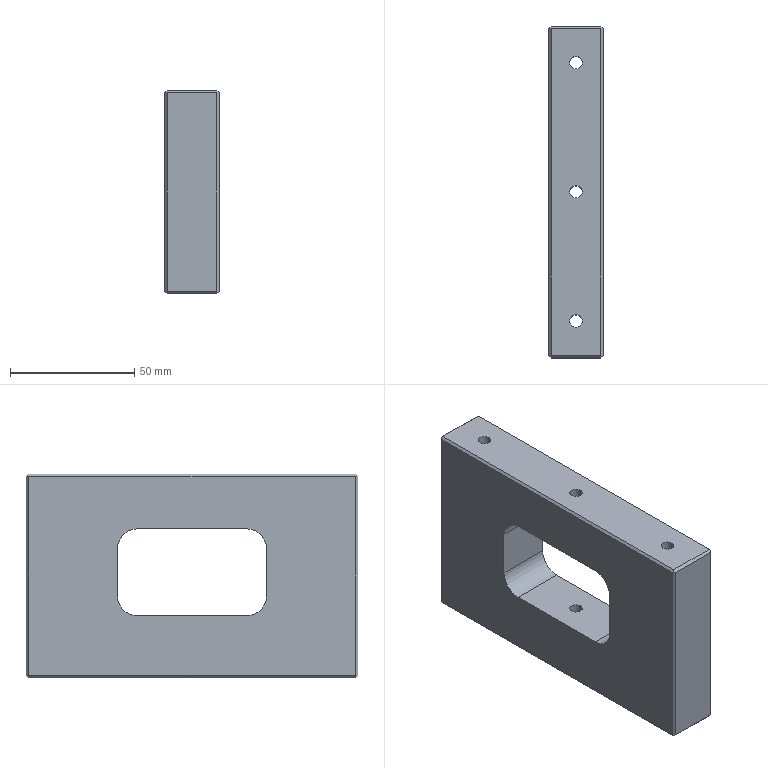Part | Creo | features DATUM PLANE 3, CURVE 2, CHAMFER 1, COORDINATE SYSTEM 1, CUT 1, PROTRUSION 1, ROUND 1 | 1 solid | 34 faces | box 22 x 133.5 x 82 mm | volume 191231 mm3 | plane 22 | cylinder 12 | commonest cylinder face diameters 5 x8 16 x4
STEP:
#1=CARTESIAN_POINT('',(0.,0.,0.));
#2=DIRECTION('',(0.,0.,1.));
#3=DIRECTION('',(1.,0.,0.));
#4=AXIS2_PLACEMENT_3D('',#1,#2,#3);
#5=CARTESIAN_POINT('',(-10.,-65.75,0.));
#6=VERTEX_POINT('',#5);
#7=CARTESIAN_POINT('',(-10.,65.75,0.));
#8=VERTEX_POINT('',#7);
#9=CARTESIAN_POINT('',(-10.,-65.75,0.));
#10=DIRECTION('',(0.,1.,0.));
#11=VECTOR('',#10,131.5);
#12=LINE('',#9,#11);
#13=EDGE_CURVE('',#6,#8,#12,.T.);
#14=ORIENTED_EDGE('',*,*,#13,.F.);
#15=CARTESIAN_POINT('',(10.,-65.75,0.));
#16=VERTEX_POINT('',#15);
#17=CARTESIAN_POINT('',(10.,-65.75,0.));
#18=DIRECTION('',(-1.,0.,0.));
#19=VECTOR('',#18,20.);
#20=LINE('',#17,#19);
#21=EDGE_CURVE('',#16,#6,#20,.T.);
#22=ORIENTED_EDGE('',*,*,#21,.F.);
#23=CARTESIAN_POINT('',(10.,65.75,0.));
#24=VERTEX_POINT('',#23);
#25=CARTESIAN_POINT('',(10.,65.75,0.));
#26=DIRECTION('',(0.,-1.,0.));
#27=VECTOR('',#26,131.5);
#28=LINE('',#25,#27);
#29=EDGE_CURVE('',#24,#16,#28,.T.);
#30=ORIENTED_EDGE('',*,*,#29,.F.);
#31=CARTESIAN_POINT('',(-10.,65.75,0.));
#32=DIRECTION('',(1.,0.,0.));
#33=VECTOR('',#32,20.);
#34=LINE('',#31,#33);
#35=EDGE_CURVE('',#8,#24,#34,.T.);
#36=ORIENTED_EDGE('',*,*,#35,.F.);
#37=EDGE_LOOP('',(#14,#22,#30,#36));
#38=FACE_OUTER_BOUND('',#37,.F.);
#39=CARTESIAN_POINT('',(2.5,0.,0.));
#40=VERTEX_POINT('',#39);
#41=CARTESIAN_POINT('',(-2.5,0.,0.));
#42=VERTEX_POINT('',#41);
#43=CARTESIAN_POINT('',(0.,0.,0.));
#44=DIRECTION('',(0.,0.,-1.));
#45=DIRECTION('',(1.,0.,0.));
#46=AXIS2_PLACEMENT_3D('',#43,#44,#45);
#47=CIRCLE('',#46,2.5);
#48=EDGE_CURVE('',#40,#42,#47,.T.);
#49=ORIENTED_EDGE('',*,*,#48,.T.);
#50=CARTESIAN_POINT('',(0.,0.,0.));
#51=DIRECTION('',(0.,0.,-1.));
#52=DIRECTION('',(-1.,0.,0.));
#53=AXIS2_PLACEMENT_3D('',#50,#51,#52);
#54=CIRCLE('',#53,2.5);
#55=EDGE_CURVE('',#42,#40,#54,.T.);
#56=ORIENTED_EDGE('',*,*,#55,.T.);
#57=EDGE_LOOP('',(#49,#56));
#58=FACE_BOUND('',#57,.F.);
#59=CARTESIAN_POINT('',(2.5,-52.,0.));
#60=VERTEX_POINT('',#59);
#61=CARTESIAN_POINT('',(-2.5,-52.,0.));
#62=VERTEX_POINT('',#61);
#63=CARTESIAN_POINT('',(0.,-52.,0.));
#64=DIRECTION('',(0.,0.,-1.));
#65=DIRECTION('',(1.,0.,0.));
#66=AXIS2_PLACEMENT_3D('',#63,#64,#65);
#67=CIRCLE('',#66,2.5);
#68=EDGE_CURVE('',#60,#62,#67,.T.);
#69=ORIENTED_EDGE('',*,*,#68,.T.);
#70=CARTESIAN_POINT('',(0.,-52.,0.));
#71=DIRECTION('',(0.,0.,-1.));
#72=DIRECTION('',(-1.,0.,0.));
#73=AXIS2_PLACEMENT_3D('',#70,#71,#72);
#74=CIRCLE('',#73,2.5);
#75=EDGE_CURVE('',#62,#60,#74,.T.);
#76=ORIENTED_EDGE('',*,*,#75,.T.);
#77=EDGE_LOOP('',(#69,#76));
#78=FACE_BOUND('',#77,.F.);
#79=CARTESIAN_POINT('',(2.5,52.,0.));
#80=VERTEX_POINT('',#79);
#81=CARTESIAN_POINT('',(-2.5,52.,0.));
#82=VERTEX_POINT('',#81);
#83=CARTESIAN_POINT('',(0.,52.,0.));
#84=DIRECTION('',(0.,0.,-1.));
#85=DIRECTION('',(1.,0.,0.));
#86=AXIS2_PLACEMENT_3D('',#83,#84,#85);
#87=CIRCLE('',#86,2.5);
#88=EDGE_CURVE('',#80,#82,#87,.T.);
#89=ORIENTED_EDGE('',*,*,#88,.T.);
#90=CARTESIAN_POINT('',(0.,52.,0.));
#91=DIRECTION('',(0.,0.,-1.));
#92=DIRECTION('',(-1.,0.,0.));
#93=AXIS2_PLACEMENT_3D('',#90,#91,#92);
#94=CIRCLE('',#93,2.5);
#95=EDGE_CURVE('',#82,#80,#94,.T.);
#96=ORIENTED_EDGE('',*,*,#95,.T.);
#97=EDGE_LOOP('',(#89,#96));
#98=FACE_BOUND('',#97,.F.);
#99=CARTESIAN_POINT('',(0.,0.,0.));
#100=DIRECTION('',(0.,0.,1.));
#101=DIRECTION('',(1.,0.,0.));
#102=AXIS2_PLACEMENT_3D('',#99,#100,#101);
#103=PLANE('',#102);
#104=ADVANCED_FACE('',(#38,#58,#78,#98),#103,.F.);
#105=ORIENTED_EDGE('',*,*,#88,.F.);
#106=CARTESIAN_POINT('',(2.5,52.,82.));
#107=VERTEX_POINT('',#106);
#108=CARTESIAN_POINT('',(2.5,52.,0.));
#109=DIRECTION('',(0.,0.,1.));
#110=VECTOR('',#109,82.);
#111=LINE('',#108,#110);
#112=EDGE_CURVE('',#80,#107,#111,.T.);
#113=ORIENTED_EDGE('',*,*,#112,.T.);
#114=CARTESIAN_POINT('',(-2.5,52.,82.));
#115=VERTEX_POINT('',#114);
#116=CARTESIAN_POINT('',(0.,52.,82.));
#117=DIRECTION('',(0.,0.,-1.));
#118=DIRECTION('',(1.,0.,0.));
#119=AXIS2_PLACEMENT_3D('',#116,#117,#118);
#120=CIRCLE('',#119,2.5);
#121=EDGE_CURVE('',#107,#115,#120,.T.);
#122=ORIENTED_EDGE('',*,*,#121,.T.);
#123=CARTESIAN_POINT('',(-2.5,52.,0.));
#124=DIRECTION('',(0.,0.,1.));
#125=VECTOR('',#124,82.);
#126=LINE('',#123,#125);
#127=EDGE_CURVE('',#82,#115,#126,.T.);
#128=ORIENTED_EDGE('',*,*,#127,.F.);
#129=EDGE_LOOP('',(#105,#113,#122,#128));
#130=FACE_OUTER_BOUND('',#129,.F.);
#131=CARTESIAN_POINT('',(0.,52.,0.));
#132=DIRECTION('',(0.,0.,1.));
#133=DIRECTION('',(1.,0.,0.));
#134=AXIS2_PLACEMENT_3D('',#131,#132,#133);
#135=CYLINDRICAL_SURFACE('',#134,2.5);
#136=ADVANCED_FACE('',(#130),#135,.F.);
#137=ORIENTED_EDGE('',*,*,#95,.F.);
#138=ORIENTED_EDGE('',*,*,#127,.T.);
#139=CARTESIAN_POINT('',(0.,52.,82.));
#140=DIRECTION('',(0.,0.,-1.));
#141=DIRECTION('',(-1.,0.,0.));
#142=AXIS2_PLACEMENT_3D('',#139,#140,#141);
#143=CIRCLE('',#142,2.5);
#144=EDGE_CURVE('',#115,#107,#143,.T.);
#145=ORIENTED_EDGE('',*,*,#144,.T.);
#146=ORIENTED_EDGE('',*,*,#112,.F.);
#147=EDGE_LOOP('',(#137,#138,#145,#146));
#148=FACE_OUTER_BOUND('',#147,.F.);
#149=CARTESIAN_POINT('',(0.,52.,0.));
#150=DIRECTION('',(0.,0.,1.));
#151=DIRECTION('',(1.,0.,0.));
#152=AXIS2_PLACEMENT_3D('',#149,#150,#151);
#153=CYLINDRICAL_SURFACE('',#152,2.5);
#154=ADVANCED_FACE('',(#148),#153,.F.);
#155=CARTESIAN_POINT('',(10.,65.75,82.));
#156=VERTEX_POINT('',#155);
#157=CARTESIAN_POINT('',(-10.,65.75,82.));
#158=VERTEX_POINT('',#157);
#159=CARTESIAN_POINT('',(10.,65.75,82.));
#160=DIRECTION('',(-1.,0.,0.));
#161=VECTOR('',#160,20.);
#162=LINE('',#159,#161);
#163=EDGE_CURVE('',#156,#158,#162,.T.);
#164=ORIENTED_EDGE('',*,*,#163,.F.);
#165=CARTESIAN_POINT('',(10.,-65.75,82.));
#166=VERTEX_POINT('',#165);
#167=CARTESIAN_POINT('',(10.,-65.75,82.));
#168=DIRECTION('',(0.,1.,0.));
#169=VECTOR('',#168,131.5);
#170=LINE('',#167,#169);
#171=EDGE_CURVE('',#166,#156,#170,.T.);
#172=ORIENTED_EDGE('',*,*,#171,.F.);
#173=CARTESIAN_POINT('',(-10.,-65.75,82.));
#174=VERTEX_POINT('',#173);
#175=CARTESIAN_POINT('',(-10.,-65.75,82.));
#176=DIRECTION('',(1.,0.,0.));
#177=VECTOR('',#176,20.);
#178=LINE('',#175,#177);
#179=EDGE_CURVE('',#174,#166,#178,.T.);
#180=ORIENTED_EDGE('',*,*,#179,.F.);
#181=CARTESIAN_POINT('',(-10.,65.75,82.));
#182=DIRECTION('',(0.,-1.,0.));
#183=VECTOR('',#182,131.5);
#184=LINE('',#181,#183);
#185=EDGE_CURVE('',#158,#174,#184,.T.);
#186=ORIENTED_EDGE('',*,*,#185,.F.);
#187=EDGE_LOOP('',(#164,#172,#180,#186));
#188=FACE_OUTER_BOUND('',#187,.F.);
#189=CARTESIAN_POINT('',(2.5,0.,82.));
#190=VERTEX_POINT('',#189);
#191=CARTESIAN_POINT('',(-2.5,0.,82.));
#192=VERTEX_POINT('',#191);
#193=CARTESIAN_POINT('',(0.,0.,82.));
#194=DIRECTION('',(0.,0.,-1.));
#195=DIRECTION('',(1.,0.,0.));
#196=AXIS2_PLACEMENT_3D('',#193,#194,#195);
#197=CIRCLE('',#196,2.5);
#198=EDGE_CURVE('',#190,#192,#197,.T.);
#199=ORIENTED_EDGE('',*,*,#198,.F.);
#200=CARTESIAN_POINT('',(0.,0.,82.));
#201=DIRECTION('',(0.,0.,-1.));
#202=DIRECTION('',(-1.,0.,0.));
#203=AXIS2_PLACEMENT_3D('',#200,#201,#202);
#204=CIRCLE('',#203,2.5);
#205=EDGE_CURVE('',#192,#190,#204,.T.);
#206=ORIENTED_EDGE('',*,*,#205,.F.);
#207=EDGE_LOOP('',(#199,#206));
#208=FACE_BOUND('',#207,.F.);
#209=CARTESIAN_POINT('',(2.5,-52.,82.));
#210=VERTEX_POINT('',#209);
#211=CARTESIAN_POINT('',(-2.5,-52.,82.));
#212=VERTEX_POINT('',#211);
#213=CARTESIAN_POINT('',(0.,-52.,82.));
#214=DIRECTION('',(0.,0.,-1.));
#215=DIRECTION('',(1.,0.,0.));
#216=AXIS2_PLACEMENT_3D('',#213,#214,#215);
#217=CIRCLE('',#216,2.5);
#218=EDGE_CURVE('',#210,#212,#217,.T.);
#219=ORIENTED_EDGE('',*,*,#218,.F.);
#220=CARTESIAN_POINT('',(0.,-52.,82.));
#221=DIRECTION('',(0.,0.,-1.));
#222=DIRECTION('',(-1.,0.,0.));
#223=AXIS2_PLACEMENT_3D('',#220,#221,#222);
#224=CIRCLE('',#223,2.5);
#225=EDGE_CURVE('',#212,#210,#224,.T.);
#226=ORIENTED_EDGE('',*,*,#225,.F.);
#227=EDGE_LOOP('',(#219,#226));
#228=FACE_BOUND('',#227,.F.);
#229=ORIENTED_EDGE('',*,*,#121,.F.);
#230=ORIENTED_EDGE('',*,*,#144,.F.);
#231=EDGE_LOOP('',(#229,#230));
#232=FACE_BOUND('',#231,.F.);
#233=CARTESIAN_POINT('',(0.,0.,82.));
#234=DIRECTION('',(0.,0.,1.));
#235=DIRECTION('',(1.,0.,0.));
#236=AXIS2_PLACEMENT_3D('',#233,#234,#235);
#237=PLANE('',#236);
#238=ADVANCED_FACE('',(#188,#208,#228,#232),#237,.T.);
#239=CARTESIAN_POINT('',(-2.5,0.,60.));
#240=VERTEX_POINT('',#239);
#241=CARTESIAN_POINT('',(2.5,0.,60.));
#242=VERTEX_POINT('',#241);
#243=CARTESIAN_POINT('',(0.,0.,60.));
#244=DIRECTION('',(0.,0.,1.));
#245=DIRECTION('',(-1.,0.,0.));
#246=AXIS2_PLACEMENT_3D('',#243,#244,#245);
#247=CIRCLE('',#246,2.5);
#248=EDGE_CURVE('',#240,#242,#247,.T.);
#249=ORIENTED_EDGE('',*,*,#248,.T.);
#250=CARTESIAN_POINT('',(2.5,0.,60.));
#251=DIRECTION('',(0.,0.,1.));
#252=VECTOR('',#251,22.);
#253=LINE('',#250,#252);
#254=EDGE_CURVE('',#242,#190,#253,.T.);
#255=ORIENTED_EDGE('',*,*,#254,.T.);
#256=ORIENTED_EDGE('',*,*,#198,.T.);
#257=CARTESIAN_POINT('',(-2.5,0.,60.));
#258=DIRECTION('',(0.,0.,1.));
#259=VECTOR('',#258,22.);
#260=LINE('',#257,#259);
#261=EDGE_CURVE('',#240,#192,#260,.T.);
#262=ORIENTED_EDGE('',*,*,#261,.F.);
#263=EDGE_LOOP('',(#249,#255,#256,#262));
#264=FACE_OUTER_BOUND('',#263,.F.);
#265=CARTESIAN_POINT('',(0.,0.,0.));
#266=DIRECTION('',(0.,0.,1.));
#267=DIRECTION('',(1.,0.,0.));
#268=AXIS2_PLACEMENT_3D('',#265,#266,#267);
#269=CYLINDRICAL_SURFACE('',#268,2.5);
#270=ADVANCED_FACE('',(#264),#269,.F.);
#271=CARTESIAN_POINT('',(-2.5,0.,25.));
#272=VERTEX_POINT('',#271);
#273=CARTESIAN_POINT('',(2.5,0.,25.));
#274=VERTEX_POINT('',#273);
#275=CARTESIAN_POINT('',(0.,0.,25.));
#276=DIRECTION('',(0.,0.,1.));
#277=DIRECTION('',(-1.,0.,0.));
#278=AXIS2_PLACEMENT_3D('',#275,#276,#277);
#279=CIRCLE('',#278,2.5);
#280=EDGE_CURVE('',#272,#274,#279,.T.);
#281=ORIENTED_EDGE('',*,*,#280,.F.);
#282=CARTESIAN_POINT('',(-2.5,0.,0.));
#283=DIRECTION('',(0.,0.,1.));
#284=VECTOR('',#283,25.);
#285=LINE('',#282,#284);
#286=EDGE_CURVE('',#42,#272,#285,.T.);
#287=ORIENTED_EDGE('',*,*,#286,.F.);
#288=ORIENTED_EDGE('',*,*,#48,.F.);
#289=CARTESIAN_POINT('',(2.5,0.,0.));
#290=DIRECTION('',(0.,0.,1.));
#291=VECTOR('',#290,25.);
#292=LINE('',#289,#291);
#293=EDGE_CURVE('',#40,#274,#292,.T.);
#294=ORIENTED_EDGE('',*,*,#293,.T.);
#295=EDGE_LOOP('',(#281,#287,#288,#294));
#296=FACE_OUTER_BOUND('',#295,.F.);
#297=CARTESIAN_POINT('',(0.,0.,0.));
#298=DIRECTION('',(0.,0.,1.));
#299=DIRECTION('',(1.,0.,0.));
#300=AXIS2_PLACEMENT_3D('',#297,#298,#299);
#301=CYLINDRICAL_SURFACE('',#300,2.5);
#302=ADVANCED_FACE('',(#296),#301,.F.);
#303=CARTESIAN_POINT('',(11.,22.,60.));
#304=VERTEX_POINT('',#303);
#305=CARTESIAN_POINT('',(-11.,22.,60.));
#306=VERTEX_POINT('',#305);
#307=CARTESIAN_POINT('',(11.,22.,60.));
#308=DIRECTION('',(-1.,0.,0.));
#309=VECTOR('',#308,22.);
#310=LINE('',#307,#309);
#311=EDGE_CURVE('',#304,#306,#310,.T.);
#312=ORIENTED_EDGE('',*,*,#311,.T.);
#313=CARTESIAN_POINT('',(-11.,-22.,60.));
#314=VERTEX_POINT('',#313);
#315=CARTESIAN_POINT('',(-11.,22.,60.));
#316=DIRECTION('',(0.,-1.,0.));
#317=VECTOR('',#316,44.);
#318=LINE('',#315,#317);
#319=EDGE_CURVE('',#306,#314,#318,.T.);
#320=ORIENTED_EDGE('',*,*,#319,.T.);
#321=CARTESIAN_POINT('',(11.,-22.,60.));
#322=VERTEX_POINT('',#321);
#323=CARTESIAN_POINT('',(11.,-22.,60.));
#324=DIRECTION('',(-1.,0.,0.));
#325=VECTOR('',#324,22.);
#326=LINE('',#323,#325);
#327=EDGE_CURVE('',#322,#314,#326,.T.);
#328=ORIENTED_EDGE('',*,*,#327,.F.);
#329=CARTESIAN_POINT('',(11.,22.,60.));
#330=DIRECTION('',(0.,-1.,0.));
#331=VECTOR('',#330,44.);
#332=LINE('',#329,#331);
#333=EDGE_CURVE('',#304,#322,#332,.T.);
#334=ORIENTED_EDGE('',*,*,#333,.F.);
#335=EDGE_LOOP('',(#312,#320,#328,#334));
#336=FACE_OUTER_BOUND('',#335,.F.);
#337=ORIENTED_EDGE('',*,*,#248,.F.);
#338=CARTESIAN_POINT('',(0.,0.,60.));
#339=DIRECTION('',(0.,0.,1.));
#340=DIRECTION('',(1.,0.,0.));
#341=AXIS2_PLACEMENT_3D('',#338,#339,#340);
#342=CIRCLE('',#341,2.5);
#343=EDGE_CURVE('',#242,#240,#342,.T.);
#344=ORIENTED_EDGE('',*,*,#343,.F.);
#345=EDGE_LOOP('',(#337,#344));
#346=FACE_BOUND('',#345,.F.);
#347=CARTESIAN_POINT('',(11.,30.,60.));
#348=DIRECTION('',(0.,0.,1.));
#349=DIRECTION('',(0.,-1.,0.));
#350=AXIS2_PLACEMENT_3D('',#347,#348,#349);
#351=PLANE('',#350);
#352=ADVANCED_FACE('',(#336,#346),#351,.F.);
#353=ORIENTED_EDGE('',*,*,#343,.T.);
#354=ORIENTED_EDGE('',*,*,#261,.T.);
#355=ORIENTED_EDGE('',*,*,#205,.T.);
#356=ORIENTED_EDGE('',*,*,#254,.F.);
#357=EDGE_LOOP('',(#353,#354,#355,#356));
#358=FACE_OUTER_BOUND('',#357,.F.);
#359=CARTESIAN_POINT('',(0.,0.,0.));
#360=DIRECTION('',(0.,0.,1.));
#361=DIRECTION('',(1.,0.,0.));
#362=AXIS2_PLACEMENT_3D('',#359,#360,#361);
#363=CYLINDRICAL_SURFACE('',#362,2.5);
#364=ADVANCED_FACE('',(#358),#363,.F.);
#365=CARTESIAN_POINT('',(0.,0.,25.));
#366=DIRECTION('',(0.,0.,1.));
#367=DIRECTION('',(1.,0.,0.));
#368=AXIS2_PLACEMENT_3D('',#365,#366,#367);
#369=CIRCLE('',#368,2.5);
#370=EDGE_CURVE('',#274,#272,#369,.T.);
#371=ORIENTED_EDGE('',*,*,#370,.F.);
#372=ORIENTED_EDGE('',*,*,#293,.F.);
#373=ORIENTED_EDGE('',*,*,#55,.F.);
#374=ORIENTED_EDGE('',*,*,#286,.T.);
#375=EDGE_LOOP('',(#371,#372,#373,#374));
#376=FACE_OUTER_BOUND('',#375,.F.);
#377=CARTESIAN_POINT('',(0.,0.,0.));
#378=DIRECTION('',(0.,0.,1.));
#379=DIRECTION('',(1.,0.,0.));
#380=AXIS2_PLACEMENT_3D('',#377,#378,#379);
#381=CYLINDRICAL_SURFACE('',#380,2.5);
#382=ADVANCED_FACE('',(#376),#381,.F.);
#383=CARTESIAN_POINT('',(11.,22.,25.));
#384=VERTEX_POINT('',#383);
#385=CARTESIAN_POINT('',(-11.,22.,25.));
#386=VERTEX_POINT('',#385);
#387=CARTESIAN_POINT('',(11.,22.,25.));
#388=DIRECTION('',(-1.,0.,0.));
#389=VECTOR('',#388,22.);
#390=LINE('',#387,#389);
#391=EDGE_CURVE('',#384,#386,#390,.T.);
#392=ORIENTED_EDGE('',*,*,#391,.F.);
#393=CARTESIAN_POINT('',(11.,-22.,25.));
#394=VERTEX_POINT('',#393);
#395=CARTESIAN_POINT('',(11.,-22.,25.));
#396=DIRECTION('',(0.,1.,0.));
#397=VECTOR('',#396,44.);
#398=LINE('',#395,#397);
#399=EDGE_CURVE('',#394,#384,#398,.T.);
#400=ORIENTED_EDGE('',*,*,#399,.F.);
#401=CARTESIAN_POINT('',(-11.,-22.,25.));
#402=VERTEX_POINT('',#401);
#403=CARTESIAN_POINT('',(11.,-22.,25.));
#404=DIRECTION('',(-1.,0.,0.));
#405=VECTOR('',#404,22.);
#406=LINE('',#403,#405);
#407=EDGE_CURVE('',#394,#402,#406,.T.);
#408=ORIENTED_EDGE('',*,*,#407,.T.);
#409=CARTESIAN_POINT('',(-11.,-22.,25.));
#410=DIRECTION('',(0.,1.,0.));
#411=VECTOR('',#410,44.);
#412=LINE('',#409,#411);
#413=EDGE_CURVE('',#402,#386,#412,.T.);
#414=ORIENTED_EDGE('',*,*,#413,.T.);
#415=EDGE_LOOP('',(#392,#400,#408,#414));
#416=FACE_OUTER_BOUND('',#415,.F.);
#417=ORIENTED_EDGE('',*,*,#280,.T.);
#418=ORIENTED_EDGE('',*,*,#370,.T.);
#419=EDGE_LOOP('',(#417,#418));
#420=FACE_BOUND('',#419,.F.);
#421=CARTESIAN_POINT('',(11.,-30.,25.));
#422=DIRECTION('',(0.,0.,-1.));
#423=DIRECTION('',(0.,1.,0.));
#424=AXIS2_PLACEMENT_3D('',#421,#422,#423);
#425=PLANE('',#424);
#426=ADVANCED_FACE('',(#416,#420),#425,.F.);
#427=CARTESIAN_POINT('',(11.,30.,33.));
#428=VERTEX_POINT('',#427);
#429=CARTESIAN_POINT('',(-11.,30.,33.));
#430=VERTEX_POINT('',#429);
#431=CARTESIAN_POINT('',(11.,30.,33.));
#432=DIRECTION('',(-1.,0.,0.));
#433=VECTOR('',#432,22.);
#434=LINE('',#431,#433);
#435=EDGE_CURVE('',#428,#430,#434,.T.);
#436=ORIENTED_EDGE('',*,*,#435,.F.);
#437=CARTESIAN_POINT('',(11.,22.,33.));
#438=DIRECTION('',(-1.,0.,0.));
#439=DIRECTION('',(0.,1.,0.));
#440=AXIS2_PLACEMENT_3D('',#437,#438,#439);
#441=CIRCLE('',#440,8.);
#442=EDGE_CURVE('',#428,#384,#441,.T.);
#443=ORIENTED_EDGE('',*,*,#442,.T.);
#444=ORIENTED_EDGE('',*,*,#391,.T.);
#445=CARTESIAN_POINT('',(-11.,22.,33.));
#446=DIRECTION('',(1.,0.,0.));
#447=DIRECTION('',(0.,0.,-1.));
#448=AXIS2_PLACEMENT_3D('',#445,#446,#447);
#449=CIRCLE('',#448,8.);
#450=EDGE_CURVE('',#386,#430,#449,.T.);
#451=ORIENTED_EDGE('',*,*,#450,.T.);
#452=EDGE_LOOP('',(#436,#443,#444,#451));
#453=FACE_OUTER_BOUND('',#452,.F.);
#454=CARTESIAN_POINT('',(39.679,22.,33.));
#455=DIRECTION('',(-1.,0.,0.));
#456=DIRECTION('',(0.,1.,0.));
#457=AXIS2_PLACEMENT_3D('',#454,#455,#456);
#458=CYLINDRICAL_SURFACE('',#457,8.);
#459=ADVANCED_FACE('',(#453),#458,.F.);
#460=CARTESIAN_POINT('',(11.,30.,52.));
#461=VERTEX_POINT('',#460);
#462=CARTESIAN_POINT('',(-11.,30.,52.));
#463=VERTEX_POINT('',#462);
#464=CARTESIAN_POINT('',(11.,30.,52.));
#465=DIRECTION('',(-1.,0.,0.));
#466=VECTOR('',#465,22.);
#467=LINE('',#464,#466);
#468=EDGE_CURVE('',#461,#463,#467,.T.);
#469=ORIENTED_EDGE('',*,*,#468,.F.);
#470=CARTESIAN_POINT('',(11.,30.,33.));
#471=DIRECTION('',(0.,0.,1.));
#472=VECTOR('',#471,19.);
#473=LINE('',#470,#472);
#474=EDGE_CURVE('',#428,#461,#473,.T.);
#475=ORIENTED_EDGE('',*,*,#474,.F.);
#476=ORIENTED_EDGE('',*,*,#435,.T.);
#477=CARTESIAN_POINT('',(-11.,30.,33.));
#478=DIRECTION('',(0.,0.,1.));
#479=VECTOR('',#478,19.);
#480=LINE('',#477,#479);
#481=EDGE_CURVE('',#430,#463,#480,.T.);
#482=ORIENTED_EDGE('',*,*,#481,.T.);
#483=EDGE_LOOP('',(#469,#475,#476,#482));
#484=FACE_OUTER_BOUND('',#483,.F.);
#485=CARTESIAN_POINT('',(11.,30.,25.));
#486=DIRECTION('',(0.,1.,0.));
#487=DIRECTION('',(0.,0.,1.));
#488=AXIS2_PLACEMENT_3D('',#485,#486,#487);
#489=PLANE('',#488);
#490=ADVANCED_FACE('',(#484),#489,.F.);
#491=ORIENTED_EDGE('',*,*,#311,.F.);
#492=CARTESIAN_POINT('',(11.,22.,52.));
#493=DIRECTION('',(-1.,0.,0.));
#494=DIRECTION('',(0.,0.,1.));
#495=AXIS2_PLACEMENT_3D('',#492,#493,#494);
#496=CIRCLE('',#495,8.);
#497=EDGE_CURVE('',#304,#461,#496,.T.);
#498=ORIENTED_EDGE('',*,*,#497,.T.);
#499=ORIENTED_EDGE('',*,*,#468,.T.);
#500=CARTESIAN_POINT('',(-11.,22.,52.));
#501=DIRECTION('',(1.,0.,0.));
#502=DIRECTION('',(0.,1.,0.));
#503=AXIS2_PLACEMENT_3D('',#500,#501,#502);
#504=CIRCLE('',#503,8.);
#505=EDGE_CURVE('',#463,#306,#504,.T.);
#506=ORIENTED_EDGE('',*,*,#505,.T.);
#507=EDGE_LOOP('',(#491,#498,#499,#506));
#508=FACE_OUTER_BOUND('',#507,.F.);
#509=CARTESIAN_POINT('',(39.679,22.,52.));
#510=DIRECTION('',(-1.,0.,0.));
#511=DIRECTION('',(0.,0.,1.));
#512=AXIS2_PLACEMENT_3D('',#509,#510,#511);
#513=CYLINDRICAL_SURFACE('',#512,8.);
#514=ADVANCED_FACE('',(#508),#513,.F.);
#515=CARTESIAN_POINT('',(11.,65.75,81.));
#516=VERTEX_POINT('',#515);
#517=CARTESIAN_POINT('',(11.,65.75,1.));
#518=VERTEX_POINT('',#517);
#519=CARTESIAN_POINT('',(11.,65.75,81.));
#520=DIRECTION('',(0.,0.,-1.));
#521=VECTOR('',#520,80.);
#522=LINE('',#519,#521);
#523=EDGE_CURVE('',#516,#518,#522,.T.);
#524=ORIENTED_EDGE('',*,*,#523,.T.);
#525=CARTESIAN_POINT('',(11.,-65.75,1.));
#526=VERTEX_POINT('',#525);
#527=CARTESIAN_POINT('',(11.,65.75,1.));
#528=DIRECTION('',(0.,-1.,0.));
#529=VECTOR('',#528,131.5);
#530=LINE('',#527,#529);
#531=EDGE_CURVE('',#518,#526,#530,.T.);
#532=ORIENTED_EDGE('',*,*,#531,.T.);
#533=CARTESIAN_POINT('',(11.,-65.75,81.));
#534=VERTEX_POINT('',#533);
#535=CARTESIAN_POINT('',(11.,-65.75,81.));
#536=DIRECTION('',(0.,0.,-1.));
#537=VECTOR('',#536,80.);
#538=LINE('',#535,#537);
#539=EDGE_CURVE('',#534,#526,#538,.T.);
#540=ORIENTED_EDGE('',*,*,#539,.F.);
#541=CARTESIAN_POINT('',(11.,-65.75,81.));
#542=DIRECTION('',(0.,1.,0.));
#543=VECTOR('',#542,131.5);
#544=LINE('',#541,#543);
#545=EDGE_CURVE('',#534,#516,#544,.T.);
#546=ORIENTED_EDGE('',*,*,#545,.T.);
#547=EDGE_LOOP('',(#524,#532,#540,#546));
#548=FACE_OUTER_BOUND('',#547,.F.);
#549=ORIENTED_EDGE('',*,*,#399,.T.);
#550=ORIENTED_EDGE('',*,*,#442,.F.);
#551=ORIENTED_EDGE('',*,*,#474,.T.);
#552=ORIENTED_EDGE('',*,*,#497,.F.);
#553=ORIENTED_EDGE('',*,*,#333,.T.);
#554=CARTESIAN_POINT('',(11.,-30.,52.));
#555=VERTEX_POINT('',#554);
#556=CARTESIAN_POINT('',(11.,-22.,52.));
#557=DIRECTION('',(-1.,0.,0.));
#558=DIRECTION('',(0.,-1.,0.));
#559=AXIS2_PLACEMENT_3D('',#556,#557,#558);
#560=CIRCLE('',#559,8.);
#561=EDGE_CURVE('',#555,#322,#560,.T.);
#562=ORIENTED_EDGE('',*,*,#561,.F.);
#563=CARTESIAN_POINT('',(11.,-30.,33.));
#564=VERTEX_POINT('',#563);
#565=CARTESIAN_POINT('',(11.,-30.,52.));
#566=DIRECTION('',(0.,0.,-1.));
#567=VECTOR('',#566,19.);
#568=LINE('',#565,#567);
#569=EDGE_CURVE('',#555,#564,#568,.T.);
#570=ORIENTED_EDGE('',*,*,#569,.T.);
#571=CARTESIAN_POINT('',(11.,-22.,33.));
#572=DIRECTION('',(-1.,0.,0.));
#573=DIRECTION('',(0.,0.,-1.));
#574=AXIS2_PLACEMENT_3D('',#571,#572,#573);
#575=CIRCLE('',#574,8.);
#576=EDGE_CURVE('',#394,#564,#575,.T.);
#577=ORIENTED_EDGE('',*,*,#576,.F.);
#578=EDGE_LOOP('',(#549,#550,#551,#552,#553,#562,#570,#577));
#579=FACE_BOUND('',#578,.F.);
#580=CARTESIAN_POINT('',(11.,-66.75,0.));
#581=DIRECTION('',(1.,0.,0.));
#582=DIRECTION('',(0.,1.,0.));
#583=AXIS2_PLACEMENT_3D('',#580,#581,#582);
#584=PLANE('',#583);
#585=ADVANCED_FACE('',(#548,#579),#584,.T.);
#586=CARTESIAN_POINT('',(10.,66.75,81.));
#587=VERTEX_POINT('',#586);
#588=CARTESIAN_POINT('',(10.,66.75,1.));
#589=VERTEX_POINT('',#588);
#590=CARTESIAN_POINT('',(10.,66.75,81.));
#591=DIRECTION('',(0.,0.,-1.));
#592=VECTOR('',#591,80.);
#593=LINE('',#590,#592);
#594=EDGE_CURVE('',#587,#589,#593,.T.);
#595=ORIENTED_EDGE('',*,*,#594,.T.);
#596=CARTESIAN_POINT('',(10.5,66.25,0.5));
#597=VERTEX_POINT('',#596);
#598=CARTESIAN_POINT('',(10.,66.75,1.));
#599=DIRECTION('',(0.5774,-0.5774,-0.5774));
#600=VECTOR('',#599,0.866);
#601=LINE('',#598,#600);
#602=EDGE_CURVE('',#589,#597,#601,.T.);
#603=ORIENTED_EDGE('',*,*,#602,.T.);
#604=CARTESIAN_POINT('',(11.,65.75,1.));
#605=DIRECTION('',(-0.5774,0.5774,-0.5774));
#606=VECTOR('',#605,0.866);
#607=LINE('',#604,#606);
#608=EDGE_CURVE('',#518,#597,#607,.T.);
#609=ORIENTED_EDGE('',*,*,#608,.F.);
#610=ORIENTED_EDGE('',*,*,#523,.F.);
#611=CARTESIAN_POINT('',(10.5,66.25,81.5));
#612=VERTEX_POINT('',#611);
#613=CARTESIAN_POINT('',(10.5,66.25,81.5));
#614=DIRECTION('',(0.5774,-0.5774,-0.5774));
#615=VECTOR('',#614,0.866);
#616=LINE('',#613,#615);
#617=EDGE_CURVE('',#612,#516,#616,.T.);
#618=ORIENTED_EDGE('',*,*,#617,.F.);
#619=CARTESIAN_POINT('',(10.,66.75,81.));
#620=DIRECTION('',(0.5774,-0.5774,0.5774));
#621=VECTOR('',#620,0.866);
#622=LINE('',#619,#621);
#623=EDGE_CURVE('',#587,#612,#622,.T.);
#624=ORIENTED_EDGE('',*,*,#623,.F.);
#625=EDGE_LOOP('',(#595,#603,#609,#610,#618,#624));
#626=FACE_OUTER_BOUND('',#625,.F.);
#627=CARTESIAN_POINT('',(10.5,66.25,41.));
#628=DIRECTION('',(0.7071,0.7071,0.));
#629=DIRECTION('',(0.7071,-0.7071,0.));
#630=AXIS2_PLACEMENT_3D('',#627,#628,#629);
#631=PLANE('',#630);
#632=ADVANCED_FACE('',(#626),#631,.T.);
#633=ORIENTED_EDGE('',*,*,#594,.F.);
#634=CARTESIAN_POINT('',(-10.,66.75,81.));
#635=VERTEX_POINT('',#634);
#636=CARTESIAN_POINT('',(10.,66.75,81.));
#637=DIRECTION('',(-1.,0.,0.));
#638=VECTOR('',#637,20.);
#639=LINE('',#636,#638);
#640=EDGE_CURVE('',#587,#635,#639,.T.);
#641=ORIENTED_EDGE('',*,*,#640,.T.);
#642=CARTESIAN_POINT('',(-10.,66.75,1.));
#643=VERTEX_POINT('',#642);
#644=CARTESIAN_POINT('',(-10.,66.75,81.));
#645=DIRECTION('',(0.,0.,-1.));
#646=VECTOR('',#645,80.);
#647=LINE('',#644,#646);
#648=EDGE_CURVE('',#635,#643,#647,.T.);
#649=ORIENTED_EDGE('',*,*,#648,.T.);
#650=CARTESIAN_POINT('',(-10.,66.75,1.));
#651=DIRECTION('',(1.,0.,0.));
#652=VECTOR('',#651,20.);
#653=LINE('',#650,#652);
#654=EDGE_CURVE('',#643,#589,#653,.T.);
#655=ORIENTED_EDGE('',*,*,#654,.T.);
#656=EDGE_LOOP('',(#633,#641,#649,#655));
#657=FACE_OUTER_BOUND('',#656,.F.);
#658=CARTESIAN_POINT('',(11.,66.75,0.));
#659=DIRECTION('',(0.,1.,0.));
#660=DIRECTION('',(-1.,0.,0.));
#661=AXIS2_PLACEMENT_3D('',#658,#659,#660);
#662=PLANE('',#661);
#663=ADVANCED_FACE('',(#657),#662,.T.);
#664=ORIENTED_EDGE('',*,*,#640,.F.);
#665=ORIENTED_EDGE('',*,*,#623,.T.);
#666=CARTESIAN_POINT('',(10.,65.75,82.));
#667=DIRECTION('',(0.5774,0.5774,-0.5774));
#668=VECTOR('',#667,0.866);
#669=LINE('',#666,#668);
#670=EDGE_CURVE('',#156,#612,#669,.T.);
#671=ORIENTED_EDGE('',*,*,#670,.F.);
#672=ORIENTED_EDGE('',*,*,#163,.T.);
#673=CARTESIAN_POINT('',(-10.5,66.25,81.5));
#674=VERTEX_POINT('',#673);
#675=CARTESIAN_POINT('',(-10.,65.75,82.));
#676=DIRECTION('',(-0.5774,0.5774,-0.5774));
#677=VECTOR('',#676,0.866);
#678=LINE('',#675,#677);
#679=EDGE_CURVE('',#158,#674,#678,.T.);
#680=ORIENTED_EDGE('',*,*,#679,.T.);
#681=CARTESIAN_POINT('',(-10.5,66.25,81.5));
#682=DIRECTION('',(0.5774,0.5774,-0.5774));
#683=VECTOR('',#682,0.866);
#684=LINE('',#681,#683);
#685=EDGE_CURVE('',#674,#635,#684,.T.);
#686=ORIENTED_EDGE('',*,*,#685,.T.);
#687=EDGE_LOOP('',(#664,#665,#671,#672,#680,#686));
#688=FACE_OUTER_BOUND('',#687,.F.);
#689=CARTESIAN_POINT('',(0.,66.25,81.5));
#690=DIRECTION('',(0.,0.7071,0.7071));
#691=DIRECTION('',(0.,0.7071,-0.7071));
#692=AXIS2_PLACEMENT_3D('',#689,#690,#691);
#693=PLANE('',#692);
#694=ADVANCED_FACE('',(#688),#693,.T.);
#695=ORIENTED_EDGE('',*,*,#545,.F.);
#696=CARTESIAN_POINT('',(10.5,-66.25,81.5));
#697=VERTEX_POINT('',#696);
#698=CARTESIAN_POINT('',(11.,-65.75,81.));
#699=DIRECTION('',(-0.5774,-0.5774,0.5774));
#700=VECTOR('',#699,0.866);
#701=LINE('',#698,#700);
#702=EDGE_CURVE('',#534,#697,#701,.T.);
#703=ORIENTED_EDGE('',*,*,#702,.T.);
#704=CARTESIAN_POINT('',(10.5,-66.25,81.5));
#705=DIRECTION('',(-0.5774,0.5774,0.5774));
#706=VECTOR('',#705,0.866);
#707=LINE('',#704,#706);
#708=EDGE_CURVE('',#697,#166,#707,.T.);
#709=ORIENTED_EDGE('',*,*,#708,.T.);
#710=ORIENTED_EDGE('',*,*,#171,.T.);
#711=ORIENTED_EDGE('',*,*,#670,.T.);
#712=ORIENTED_EDGE('',*,*,#617,.T.);
#713=EDGE_LOOP('',(#695,#703,#709,#710,#711,#712));
#714=FACE_OUTER_BOUND('',#713,.F.);
#715=CARTESIAN_POINT('',(10.5,0.,81.5));
#716=DIRECTION('',(0.7071,0.,0.7071));
#717=DIRECTION('',(0.7071,0.,-0.7071));
#718=AXIS2_PLACEMENT_3D('',#715,#716,#717);
#719=PLANE('',#718);
#720=ADVANCED_FACE('',(#714),#719,.T.);
#721=ORIENTED_EDGE('',*,*,#539,.T.);
#722=CARTESIAN_POINT('',(10.5,-66.25,0.5));
#723=VERTEX_POINT('',#722);
#724=CARTESIAN_POINT('',(10.5,-66.25,0.5));
#725=DIRECTION('',(0.5774,0.5774,0.5774));
#726=VECTOR('',#725,0.866);
#727=LINE('',#724,#726);
#728=EDGE_CURVE('',#723,#526,#727,.T.);
#729=ORIENTED_EDGE('',*,*,#728,.F.);
#730=CARTESIAN_POINT('',(10.,-66.75,1.));
#731=VERTEX_POINT('',#730);
#732=CARTESIAN_POINT('',(10.,-66.75,1.));
#733=DIRECTION('',(0.5774,0.5774,-0.5774));
#734=VECTOR('',#733,0.866);
#735=LINE('',#732,#734);
#736=EDGE_CURVE('',#731,#723,#735,.T.);
#737=ORIENTED_EDGE('',*,*,#736,.F.);
#738=CARTESIAN_POINT('',(10.,-66.75,81.));
#739=VERTEX_POINT('',#738);
#740=CARTESIAN_POINT('',(10.,-66.75,81.));
#741=DIRECTION('',(0.,0.,-1.));
#742=VECTOR('',#741,80.);
#743=LINE('',#740,#742);
#744=EDGE_CURVE('',#739,#731,#743,.T.);
#745=ORIENTED_EDGE('',*,*,#744,.F.);
#746=CARTESIAN_POINT('',(10.,-66.75,81.));
#747=DIRECTION('',(0.5774,0.5774,0.5774));
#748=VECTOR('',#747,0.866);
#749=LINE('',#746,#748);
#750=EDGE_CURVE('',#739,#697,#749,.T.);
#751=ORIENTED_EDGE('',*,*,#750,.T.);
#752=ORIENTED_EDGE('',*,*,#702,.F.);
#753=EDGE_LOOP('',(#721,#729,#737,#745,#751,#752));
#754=FACE_OUTER_BOUND('',#753,.F.);
#755=CARTESIAN_POINT('',(10.5,-66.25,41.));
#756=DIRECTION('',(0.7071,-0.7071,0.));
#757=DIRECTION('',(-0.7071,-0.7071,0.));
#758=AXIS2_PLACEMENT_3D('',#755,#756,#757);
#759=PLANE('',#758);
#760=ADVANCED_FACE('',(#754),#759,.T.);
#761=ORIENTED_EDGE('',*,*,#531,.F.);
#762=ORIENTED_EDGE('',*,*,#608,.T.);
#763=CARTESIAN_POINT('',(10.5,66.25,0.5));
#764=DIRECTION('',(-0.5774,-0.5774,-0.5774));
#765=VECTOR('',#764,0.866);
#766=LINE('',#763,#765);
#767=EDGE_CURVE('',#597,#24,#766,.T.);
#768=ORIENTED_EDGE('',*,*,#767,.T.);
#769=ORIENTED_EDGE('',*,*,#29,.T.);
#770=CARTESIAN_POINT('',(10.,-65.75,0.));
#771=DIRECTION('',(0.5774,-0.5774,0.5774));
#772=VECTOR('',#771,0.866);
#773=LINE('',#770,#772);
#774=EDGE_CURVE('',#16,#723,#773,.T.);
#775=ORIENTED_EDGE('',*,*,#774,.T.);
#776=ORIENTED_EDGE('',*,*,#728,.T.);
#777=EDGE_LOOP('',(#761,#762,#768,#769,#775,#776));
#778=FACE_OUTER_BOUND('',#777,.F.);
#779=CARTESIAN_POINT('',(10.5,0.,0.5));
#780=DIRECTION('',(0.7071,0.,-0.7071));
#781=DIRECTION('',(0.7071,0.,0.7071));
#782=AXIS2_PLACEMENT_3D('',#779,#780,#781);
#783=PLANE('',#782);
#784=ADVANCED_FACE('',(#778),#783,.T.);
#785=ORIENTED_EDGE('',*,*,#35,.T.);
#786=ORIENTED_EDGE('',*,*,#767,.F.);
#787=ORIENTED_EDGE('',*,*,#602,.F.);
#788=ORIENTED_EDGE('',*,*,#654,.F.);
#789=CARTESIAN_POINT('',(-10.5,66.25,0.5));
#790=VERTEX_POINT('',#789);
#791=CARTESIAN_POINT('',(-10.,66.75,1.));
#792=DIRECTION('',(-0.5774,-0.5774,-0.5774));
#793=VECTOR('',#792,0.866);
#794=LINE('',#791,#793);
#795=EDGE_CURVE('',#643,#790,#794,.T.);
#796=ORIENTED_EDGE('',*,*,#795,.T.);
#797=CARTESIAN_POINT('',(-10.5,66.25,0.5));
#798=DIRECTION('',(0.5774,-0.5774,-0.5774));
#799=VECTOR('',#798,0.866);
#800=LINE('',#797,#799);
#801=EDGE_CURVE('',#790,#8,#800,.T.);
#802=ORIENTED_EDGE('',*,*,#801,.T.);
#803=EDGE_LOOP('',(#785,#786,#787,#788,#796,#802));
#804=FACE_OUTER_BOUND('',#803,.F.);
#805=CARTESIAN_POINT('',(0.,66.25,0.5));
#806=DIRECTION('',(0.,0.7071,-0.7071));
#807=DIRECTION('',(0.,0.7071,0.7071));
#808=AXIS2_PLACEMENT_3D('',#805,#806,#807);
#809=PLANE('',#808);
#810=ADVANCED_FACE('',(#804),#809,.T.);
#811=CARTESIAN_POINT('',(-11.,65.75,81.));
#812=VERTEX_POINT('',#811);
#813=CARTESIAN_POINT('',(-11.,65.75,1.));
#814=VERTEX_POINT('',#813);
#815=CARTESIAN_POINT('',(-11.,65.75,81.));
#816=DIRECTION('',(0.,0.,-1.));
#817=VECTOR('',#816,80.);
#818=LINE('',#815,#817);
#819=EDGE_CURVE('',#812,#814,#818,.T.);
#820=ORIENTED_EDGE('',*,*,#819,.T.);
#821=CARTESIAN_POINT('',(-11.,65.75,1.));
#822=DIRECTION('',(0.5774,0.5774,-0.5774));
#823=VECTOR('',#822,0.866);
#824=LINE('',#821,#823);
#825=EDGE_CURVE('',#814,#790,#824,.T.);
#826=ORIENTED_EDGE('',*,*,#825,.T.);
#827=ORIENTED_EDGE('',*,*,#795,.F.);
#828=ORIENTED_EDGE('',*,*,#648,.F.);
#829=ORIENTED_EDGE('',*,*,#685,.F.);
#830=CARTESIAN_POINT('',(-11.,65.75,81.));
#831=DIRECTION('',(0.5774,0.5774,0.5774));
#832=VECTOR('',#831,0.866);
#833=LINE('',#830,#832);
#834=EDGE_CURVE('',#812,#674,#833,.T.);
#835=ORIENTED_EDGE('',*,*,#834,.F.);
#836=EDGE_LOOP('',(#820,#826,#827,#828,#829,#835));
#837=FACE_OUTER_BOUND('',#836,.F.);
#838=CARTESIAN_POINT('',(-10.5,66.25,41.));
#839=DIRECTION('',(-0.7071,0.7071,0.));
#840=DIRECTION('',(0.7071,0.7071,0.));
#841=AXIS2_PLACEMENT_3D('',#838,#839,#840);
#842=PLANE('',#841);
#843=ADVANCED_FACE('',(#837),#842,.T.);
#844=CARTESIAN_POINT('',(-11.,-65.75,81.));
#845=VERTEX_POINT('',#844);
#846=CARTESIAN_POINT('',(-11.,65.75,81.));
#847=DIRECTION('',(0.,-1.,0.));
#848=VECTOR('',#847,131.5);
#849=LINE('',#846,#848);
#850=EDGE_CURVE('',#812,#845,#849,.T.);
#851=ORIENTED_EDGE('',*,*,#850,.T.);
#852=CARTESIAN_POINT('',(-11.,-65.75,1.));
#853=VERTEX_POINT('',#852);
#854=CARTESIAN_POINT('',(-11.,-65.75,81.));
#855=DIRECTION('',(0.,0.,-1.));
#856=VECTOR('',#855,80.);
#857=LINE('',#854,#856);
#858=EDGE_CURVE('',#845,#853,#857,.T.);
#859=ORIENTED_EDGE('',*,*,#858,.T.);
#860=CARTESIAN_POINT('',(-11.,-65.75,1.));
#861=DIRECTION('',(0.,1.,0.));
#862=VECTOR('',#861,131.5);
#863=LINE('',#860,#862);
#864=EDGE_CURVE('',#853,#814,#863,.T.);
#865=ORIENTED_EDGE('',*,*,#864,.T.);
#866=ORIENTED_EDGE('',*,*,#819,.F.);
#867=EDGE_LOOP('',(#851,#859,#865,#866));
#868=FACE_OUTER_BOUND('',#867,.F.);
#869=ORIENTED_EDGE('',*,*,#481,.F.);
#870=ORIENTED_EDGE('',*,*,#450,.F.);
#871=ORIENTED_EDGE('',*,*,#413,.F.);
#872=CARTESIAN_POINT('',(-11.,-30.,33.));
#873=VERTEX_POINT('',#872);
#874=CARTESIAN_POINT('',(-11.,-22.,33.));
#875=DIRECTION('',(1.,0.,0.));
#876=DIRECTION('',(0.,-1.,0.));
#877=AXIS2_PLACEMENT_3D('',#874,#875,#876);
#878=CIRCLE('',#877,8.);
#879=EDGE_CURVE('',#873,#402,#878,.T.);
#880=ORIENTED_EDGE('',*,*,#879,.F.);
#881=CARTESIAN_POINT('',(-11.,-30.,52.));
#882=VERTEX_POINT('',#881);
#883=CARTESIAN_POINT('',(-11.,-30.,52.));
#884=DIRECTION('',(0.,0.,-1.));
#885=VECTOR('',#884,19.);
#886=LINE('',#883,#885);
#887=EDGE_CURVE('',#882,#873,#886,.T.);
#888=ORIENTED_EDGE('',*,*,#887,.F.);
#889=CARTESIAN_POINT('',(-11.,-22.,52.));
#890=DIRECTION('',(1.,0.,0.));
#891=DIRECTION('',(0.,0.,1.));
#892=AXIS2_PLACEMENT_3D('',#889,#890,#891);
#893=CIRCLE('',#892,8.);
#894=EDGE_CURVE('',#314,#882,#893,.T.);
#895=ORIENTED_EDGE('',*,*,#894,.F.);
#896=ORIENTED_EDGE('',*,*,#319,.F.);
#897=ORIENTED_EDGE('',*,*,#505,.F.);
#898=EDGE_LOOP('',(#869,#870,#871,#880,#888,#895,#896,#897));
#899=FACE_BOUND('',#898,.F.);
#900=CARTESIAN_POINT('',(-11.,66.75,0.));
#901=DIRECTION('',(-1.,0.,0.));
#902=DIRECTION('',(0.,-1.,0.));
#903=AXIS2_PLACEMENT_3D('',#900,#901,#902);
#904=PLANE('',#903);
#905=ADVANCED_FACE('',(#868,#899),#904,.T.);
#906=ORIENTED_EDGE('',*,*,#850,.F.);
#907=ORIENTED_EDGE('',*,*,#834,.T.);
#908=ORIENTED_EDGE('',*,*,#679,.F.);
#909=ORIENTED_EDGE('',*,*,#185,.T.);
#910=CARTESIAN_POINT('',(-10.5,-66.25,81.5));
#911=VERTEX_POINT('',#910);
#912=CARTESIAN_POINT('',(-10.,-65.75,82.));
#913=DIRECTION('',(-0.5774,-0.5774,-0.5774));
#914=VECTOR('',#913,0.866);
#915=LINE('',#912,#914);
#916=EDGE_CURVE('',#174,#911,#915,.T.);
#917=ORIENTED_EDGE('',*,*,#916,.T.);
#918=CARTESIAN_POINT('',(-10.5,-66.25,81.5));
#919=DIRECTION('',(-0.5774,0.5774,-0.5774));
#920=VECTOR('',#919,0.866);
#921=LINE('',#918,#920);
#922=EDGE_CURVE('',#911,#845,#921,.T.);
#923=ORIENTED_EDGE('',*,*,#922,.T.);
#924=EDGE_LOOP('',(#906,#907,#908,#909,#917,#923));
#925=FACE_OUTER_BOUND('',#924,.F.);
#926=CARTESIAN_POINT('',(-10.5,0.,81.5));
#927=DIRECTION('',(-0.7071,0.,0.7071));
#928=DIRECTION('',(-0.7071,0.,-0.7071));
#929=AXIS2_PLACEMENT_3D('',#926,#927,#928);
#930=PLANE('',#929);
#931=ADVANCED_FACE('',(#925),#930,.T.);
#932=ORIENTED_EDGE('',*,*,#179,.T.);
#933=ORIENTED_EDGE('',*,*,#708,.F.);
#934=ORIENTED_EDGE('',*,*,#750,.F.);
#935=CARTESIAN_POINT('',(-10.,-66.75,81.));
#936=VERTEX_POINT('',#935);
#937=CARTESIAN_POINT('',(-10.,-66.75,81.));
#938=DIRECTION('',(1.,0.,0.));
#939=VECTOR('',#938,20.);
#940=LINE('',#937,#939);
#941=EDGE_CURVE('',#936,#739,#940,.T.);
#942=ORIENTED_EDGE('',*,*,#941,.F.);
#943=CARTESIAN_POINT('',(-10.,-66.75,81.));
#944=DIRECTION('',(-0.5774,0.5774,0.5774));
#945=VECTOR('',#944,0.866);
#946=LINE('',#943,#945);
#947=EDGE_CURVE('',#936,#911,#946,.T.);
#948=ORIENTED_EDGE('',*,*,#947,.T.);
#949=ORIENTED_EDGE('',*,*,#916,.F.);
#950=EDGE_LOOP('',(#932,#933,#934,#942,#948,#949));
#951=FACE_OUTER_BOUND('',#950,.F.);
#952=CARTESIAN_POINT('',(0.,-66.25,81.5));
#953=DIRECTION('',(0.,-0.7071,0.7071));
#954=DIRECTION('',(0.,-0.7071,-0.7071));
#955=AXIS2_PLACEMENT_3D('',#952,#953,#954);
#956=PLANE('',#955);
#957=ADVANCED_FACE('',(#951),#956,.T.);
#958=ORIENTED_EDGE('',*,*,#744,.T.);
#959=CARTESIAN_POINT('',(-10.,-66.75,1.));
#960=VERTEX_POINT('',#959);
#961=CARTESIAN_POINT('',(10.,-66.75,1.));
#962=DIRECTION('',(-1.,0.,0.));
#963=VECTOR('',#962,20.);
#964=LINE('',#961,#963);
#965=EDGE_CURVE('',#731,#960,#964,.T.);
#966=ORIENTED_EDGE('',*,*,#965,.T.);
#967=CARTESIAN_POINT('',(-10.,-66.75,81.));
#968=DIRECTION('',(0.,0.,-1.));
#969=VECTOR('',#968,80.);
#970=LINE('',#967,#969);
#971=EDGE_CURVE('',#936,#960,#970,.T.);
#972=ORIENTED_EDGE('',*,*,#971,.F.);
#973=ORIENTED_EDGE('',*,*,#941,.T.);
#974=EDGE_LOOP('',(#958,#966,#972,#973));
#975=FACE_OUTER_BOUND('',#974,.F.);
#976=CARTESIAN_POINT('',(-11.,-66.75,0.));
#977=DIRECTION('',(0.,-1.,0.));
#978=DIRECTION('',(1.,0.,0.));
#979=AXIS2_PLACEMENT_3D('',#976,#977,#978);
#980=PLANE('',#979);
#981=ADVANCED_FACE('',(#975),#980,.T.);
#982=ORIENTED_EDGE('',*,*,#965,.F.);
#983=ORIENTED_EDGE('',*,*,#736,.T.);
#984=ORIENTED_EDGE('',*,*,#774,.F.);
#985=ORIENTED_EDGE('',*,*,#21,.T.);
#986=CARTESIAN_POINT('',(-10.5,-66.25,0.5));
#987=VERTEX_POINT('',#986);
#988=CARTESIAN_POINT('',(-10.5,-66.25,0.5));
#989=DIRECTION('',(0.5774,0.5774,-0.5774));
#990=VECTOR('',#989,0.866);
#991=LINE('',#988,#990);
#992=EDGE_CURVE('',#987,#6,#991,.T.);
#993=ORIENTED_EDGE('',*,*,#992,.F.);
#994=CARTESIAN_POINT('',(-10.,-66.75,1.));
#995=DIRECTION('',(-0.5774,0.5774,-0.5774));
#996=VECTOR('',#995,0.866);
#997=LINE('',#994,#996);
#998=EDGE_CURVE('',#960,#987,#997,.T.);
#999=ORIENTED_EDGE('',*,*,#998,.F.);
#1000=EDGE_LOOP('',(#982,#983,#984,#985,#993,#999));
#1001=FACE_OUTER_BOUND('',#1000,.F.);
#1002=CARTESIAN_POINT('',(0.,-66.25,0.5));
#1003=DIRECTION('',(0.,-0.7071,-0.7071));
#1004=DIRECTION('',(0.,-0.7071,0.7071));
#1005=AXIS2_PLACEMENT_3D('',#1002,#1003,#1004);
#1006=PLANE('',#1005);
#1007=ADVANCED_FACE('',(#1001),#1006,.T.);
#1008=ORIENTED_EDGE('',*,*,#13,.T.);
#1009=ORIENTED_EDGE('',*,*,#801,.F.);
#1010=ORIENTED_EDGE('',*,*,#825,.F.);
#1011=ORIENTED_EDGE('',*,*,#864,.F.);
#1012=CARTESIAN_POINT('',(-11.,-65.75,1.));
#1013=DIRECTION('',(0.5774,-0.5774,-0.5774));
#1014=VECTOR('',#1013,0.866);
#1015=LINE('',#1012,#1014);
#1016=EDGE_CURVE('',#853,#987,#1015,.T.);
#1017=ORIENTED_EDGE('',*,*,#1016,.T.);
#1018=ORIENTED_EDGE('',*,*,#992,.T.);
#1019=EDGE_LOOP('',(#1008,#1009,#1010,#1011,#1017,#1018));
#1020=FACE_OUTER_BOUND('',#1019,.F.);
#1021=CARTESIAN_POINT('',(-10.5,0.,0.5));
#1022=DIRECTION('',(-0.7071,0.,-0.7071));
#1023=DIRECTION('',(-0.7071,0.,0.7071));
#1024=AXIS2_PLACEMENT_3D('',#1021,#1022,#1023);
#1025=PLANE('',#1024);
#1026=ADVANCED_FACE('',(#1020),#1025,.T.);
#1027=ORIENTED_EDGE('',*,*,#971,.T.);
#1028=ORIENTED_EDGE('',*,*,#998,.T.);
#1029=ORIENTED_EDGE('',*,*,#1016,.F.);
#1030=ORIENTED_EDGE('',*,*,#858,.F.);
#1031=ORIENTED_EDGE('',*,*,#922,.F.);
#1032=ORIENTED_EDGE('',*,*,#947,.F.);
#1033=EDGE_LOOP('',(#1027,#1028,#1029,#1030,#1031,#1032));
#1034=FACE_OUTER_BOUND('',#1033,.F.);
#1035=CARTESIAN_POINT('',(-10.5,-66.25,41.));
#1036=DIRECTION('',(-0.7071,-0.7071,0.));
#1037=DIRECTION('',(-0.7071,0.7071,0.));
#1038=AXIS2_PLACEMENT_3D('',#1035,#1036,#1037);
#1039=PLANE('',#1038);
#1040=ADVANCED_FACE('',(#1034),#1039,.T.);
#1041=ORIENTED_EDGE('',*,*,#407,.F.);
#1042=ORIENTED_EDGE('',*,*,#576,.T.);
#1043=CARTESIAN_POINT('',(11.,-30.,33.));
#1044=DIRECTION('',(-1.,0.,0.));
#1045=VECTOR('',#1044,22.);
#1046=LINE('',#1043,#1045);
#1047=EDGE_CURVE('',#564,#873,#1046,.T.);
#1048=ORIENTED_EDGE('',*,*,#1047,.T.);
#1049=ORIENTED_EDGE('',*,*,#879,.T.);
#1050=EDGE_LOOP('',(#1041,#1042,#1048,#1049));
#1051=FACE_OUTER_BOUND('',#1050,.F.);
#1052=CARTESIAN_POINT('',(39.679,-22.,33.));
#1053=DIRECTION('',(-1.,0.,0.));
#1054=DIRECTION('',(0.,0.,-1.));
#1055=AXIS2_PLACEMENT_3D('',#1052,#1053,#1054);
#1056=CYLINDRICAL_SURFACE('',#1055,8.);
#1057=ADVANCED_FACE('',(#1051),#1056,.F.);
#1058=ORIENTED_EDGE('',*,*,#1047,.F.);
#1059=ORIENTED_EDGE('',*,*,#569,.F.);
#1060=CARTESIAN_POINT('',(11.,-30.,52.));
#1061=DIRECTION('',(-1.,0.,0.));
#1062=VECTOR('',#1061,22.);
#1063=LINE('',#1060,#1062);
#1064=EDGE_CURVE('',#555,#882,#1063,.T.);
#1065=ORIENTED_EDGE('',*,*,#1064,.T.);
#1066=ORIENTED_EDGE('',*,*,#887,.T.);
#1067=EDGE_LOOP('',(#1058,#1059,#1065,#1066));
#1068=FACE_OUTER_BOUND('',#1067,.F.);
#1069=CARTESIAN_POINT('',(11.,-30.,60.));
#1070=DIRECTION('',(0.,-1.,0.));
#1071=DIRECTION('',(0.,0.,-1.));
#1072=AXIS2_PLACEMENT_3D('',#1069,#1070,#1071);
#1073=PLANE('',#1072);
#1074=ADVANCED_FACE('',(#1068),#1073,.F.);
#1075=ORIENTED_EDGE('',*,*,#1064,.F.);
#1076=ORIENTED_EDGE('',*,*,#561,.T.);
#1077=ORIENTED_EDGE('',*,*,#327,.T.);
#1078=ORIENTED_EDGE('',*,*,#894,.T.);
#1079=EDGE_LOOP('',(#1075,#1076,#1077,#1078));
#1080=FACE_OUTER_BOUND('',#1079,.F.);
#1081=CARTESIAN_POINT('',(39.679,-22.,52.));
#1082=DIRECTION('',(-1.,0.,0.));
#1083=DIRECTION('',(0.,-1.,0.));
#1084=AXIS2_PLACEMENT_3D('',#1081,#1082,#1083);
#1085=CYLINDRICAL_SURFACE('',#1084,8.);
#1086=ADVANCED_FACE('',(#1080),#1085,.F.);
#1087=ORIENTED_EDGE('',*,*,#68,.F.);
#1088=CARTESIAN_POINT('',(2.5,-52.,0.));
#1089=DIRECTION('',(0.,0.,1.));
#1090=VECTOR('',#1089,82.);
#1091=LINE('',#1088,#1090);
#1092=EDGE_CURVE('',#60,#210,#1091,.T.);
#1093=ORIENTED_EDGE('',*,*,#1092,.T.);
#1094=ORIENTED_EDGE('',*,*,#218,.T.);
#1095=CARTESIAN_POINT('',(-2.5,-52.,0.));
#1096=DIRECTION('',(0.,0.,1.));
#1097=VECTOR('',#1096,82.);
#1098=LINE('',#1095,#1097);
#1099=EDGE_CURVE('',#62,#212,#1098,.T.);
#1100=ORIENTED_EDGE('',*,*,#1099,.F.);
#1101=EDGE_LOOP('',(#1087,#1093,#1094,#1100));
#1102=FACE_OUTER_BOUND('',#1101,.F.);
#1103=CARTESIAN_POINT('',(0.,-52.,0.));
#1104=DIRECTION('',(0.,0.,1.));
#1105=DIRECTION('',(1.,0.,0.));
#1106=AXIS2_PLACEMENT_3D('',#1103,#1104,#1105);
#1107=CYLINDRICAL_SURFACE('',#1106,2.5);
#1108=ADVANCED_FACE('',(#1102),#1107,.F.);
#1109=ORIENTED_EDGE('',*,*,#75,.F.);
#1110=ORIENTED_EDGE('',*,*,#1099,.T.);
#1111=ORIENTED_EDGE('',*,*,#225,.T.);
#1112=ORIENTED_EDGE('',*,*,#1092,.F.);
#1113=EDGE_LOOP('',(#1109,#1110,#1111,#1112));
#1114=FACE_OUTER_BOUND('',#1113,.F.);
#1115=CARTESIAN_POINT('',(0.,-52.,0.));
#1116=DIRECTION('',(0.,0.,1.));
#1117=DIRECTION('',(1.,0.,0.));
#1118=AXIS2_PLACEMENT_3D('',#1115,#1116,#1117);
#1119=CYLINDRICAL_SURFACE('',#1118,2.5);
#1120=ADVANCED_FACE('',(#1114),#1119,.F.);
#1121=CLOSED_SHELL('',(#104,#136,#154,#238,#270,#302,#352,#364,#382,#426,#459,#490,#514,#585,#632,#663,#694,#720,#760,#784,#810,#843,#905,#931,#957,#981,#1007,#1026,#1040,#1057,#1074,#1086,#1108,#1120));
#1122=MANIFOLD_SOLID_BREP('',#1121);
#1123=(LENGTH_UNIT()NAMED_UNIT(*)SI_UNIT(.MILLI.,.METRE.));
#1124=UNCERTAINTY_MEASURE_WITH_UNIT(LENGTH_MEASURE(0.01582),#1123,'','');
#1125=(NAMED_UNIT(*)PLANE_ANGLE_UNIT()SI_UNIT($,.RADIAN.));
#1126=PLANE_ANGLE_MEASURE_WITH_UNIT(PLANE_ANGLE_MEASURE(0.01745),#1125);
#1127=(CONVERSION_BASED_UNIT('DEGREE',#1126)NAMED_UNIT(*)PLANE_ANGLE_UNIT());
#1128=(NAMED_UNIT(*)SI_UNIT($,.STERADIAN.)SOLID_ANGLE_UNIT());
#1129=(GEOMETRIC_REPRESENTATION_CONTEXT(3)GLOBAL_UNCERTAINTY_ASSIGNED_CONTEXT((#1124))GLOBAL_UNIT_ASSIGNED_CONTEXT((#1123,#1127,#1128))REPRESENTATION_CONTEXT('',''));
#1130=ADVANCED_BREP_SHAPE_REPRESENTATION('',(#4,#1122),#1129);